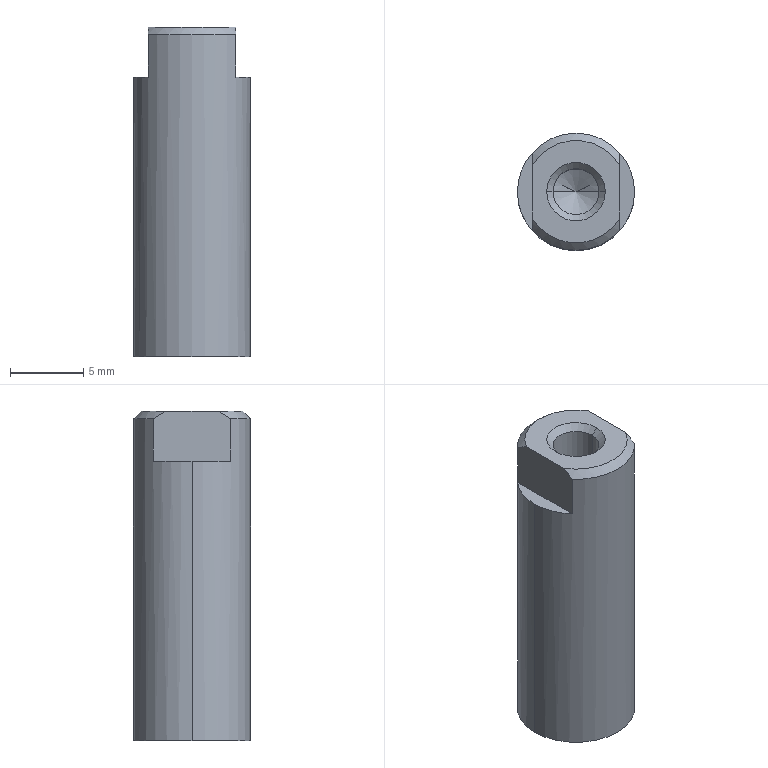Part | SolidWorks | features ICE 1, RevCut 1, Revolution 1 | 1 solid | 16 faces | box 8 x 8 x 22.5 mm | volume 1035 mm3 | cone 6 | plane 6 | cylinder 4 | commonest cylinder face diameters 3.14 x2 8 x2
STEP:
#1=CARTESIAN_POINT('',(0.,0.,-5.906));
#2=VERTEX_POINT('',#1);
#3=CARTESIAN_POINT('',(1.57,0.,-5.));
#4=VERTEX_POINT('',#3);
#5=CARTESIAN_POINT('',(0.,0.,-5.906));
#6=DIRECTION('',(0.866,0.,0.5));
#7=VECTOR('',#6,1000.);
#8=LINE('',#5,#7);
#9=EDGE_CURVE('',#2,#4,#8,.T.);
#10=ORIENTED_EDGE('',*,*,#9,.F.);
#11=CARTESIAN_POINT('',(-1.57,0.,-5.));
#12=VERTEX_POINT('',#11);
#13=CARTESIAN_POINT('',(0.,0.,-5.906));
#14=DIRECTION('',(-0.866,0.,0.5));
#15=VECTOR('',#14,1000.);
#16=LINE('',#13,#15);
#17=EDGE_CURVE('',#2,#12,#16,.T.);
#18=ORIENTED_EDGE('',*,*,#17,.T.);
#19=CARTESIAN_POINT('',(0.,0.,-5.));
#20=DIRECTION('',(0.,0.,1.));
#21=DIRECTION('',(1.,0.,0.));
#22=AXIS2_PLACEMENT_3D('',#19,#20,#21);
#23=CIRCLE('',#22,1.57);
#24=EDGE_CURVE('',#12,#4,#23,.T.);
#25=ORIENTED_EDGE('',*,*,#24,.T.);
#26=EDGE_LOOP('',(#10,#18,#25));
#27=FACE_OUTER_BOUND('',#26,.T.);
#28=CARTESIAN_POINT('',(0.,0.,994.094));
#29=DIRECTION('',(0.,0.,1.));
#30=DIRECTION('',(1.,0.,0.));
#31=AXIS2_PLACEMENT_3D('',#28,#29,#30);
#32=CONICAL_SURFACE('',#31,1732.051,1.047);
#33=ADVANCED_FACE('',(#27),#32,.F.);
#34=ORIENTED_EDGE('',*,*,#24,.F.);
#35=CARTESIAN_POINT('',(-1.57,0.,3.07));
#36=VERTEX_POINT('',#35);
#37=CARTESIAN_POINT('',(-1.57,0.,-5.906));
#38=DIRECTION('',(0.,0.,1.));
#39=VECTOR('',#38,1000.);
#40=LINE('',#37,#39);
#41=EDGE_CURVE('',#12,#36,#40,.T.);
#42=ORIENTED_EDGE('',*,*,#41,.T.);
#43=CARTESIAN_POINT('',(1.57,0.,3.07));
#44=VERTEX_POINT('',#43);
#45=CARTESIAN_POINT('',(0.,0.,3.07));
#46=DIRECTION('',(0.,0.,1.));
#47=DIRECTION('',(1.,0.,0.));
#48=AXIS2_PLACEMENT_3D('',#45,#46,#47);
#49=CIRCLE('',#48,1.57);
#50=EDGE_CURVE('',#36,#44,#49,.T.);
#51=ORIENTED_EDGE('',*,*,#50,.T.);
#52=CARTESIAN_POINT('',(1.57,0.,-5.906));
#53=DIRECTION('',(0.,0.,1.));
#54=VECTOR('',#53,1000.);
#55=LINE('',#52,#54);
#56=EDGE_CURVE('',#4,#44,#55,.T.);
#57=ORIENTED_EDGE('',*,*,#56,.F.);
#58=EDGE_LOOP('',(#34,#42,#51,#57));
#59=FACE_OUTER_BOUND('',#58,.T.);
#60=CARTESIAN_POINT('',(0.,0.,-5.906));
#61=DIRECTION('',(0.,0.,1.));
#62=DIRECTION('',(1.,0.,0.));
#63=AXIS2_PLACEMENT_3D('',#60,#61,#62);
#64=CYLINDRICAL_SURFACE('',#63,1.57);
#65=ADVANCED_FACE('',(#59),#64,.F.);
#66=ORIENTED_EDGE('',*,*,#50,.F.);
#67=CARTESIAN_POINT('',(-2.,0.,3.5));
#68=VERTEX_POINT('',#67);
#69=CARTESIAN_POINT('',(-1.57,0.,3.07));
#70=DIRECTION('',(-0.7071,0.,0.7071));
#71=VECTOR('',#70,1000.);
#72=LINE('',#69,#71);
#73=EDGE_CURVE('',#36,#68,#72,.T.);
#74=ORIENTED_EDGE('',*,*,#73,.T.);
#75=CARTESIAN_POINT('',(2.,0.,3.5));
#76=VERTEX_POINT('',#75);
#77=CARTESIAN_POINT('',(0.,0.,3.5));
#78=DIRECTION('',(0.,0.,1.));
#79=DIRECTION('',(-1.,0.,0.));
#80=AXIS2_PLACEMENT_3D('',#77,#78,#79);
#81=CIRCLE('',#80,2.);
#82=EDGE_CURVE('',#68,#76,#81,.T.);
#83=ORIENTED_EDGE('',*,*,#82,.T.);
#84=CARTESIAN_POINT('',(1.57,0.,3.07));
#85=DIRECTION('',(0.7071,0.,0.7071));
#86=VECTOR('',#85,1000.);
#87=LINE('',#84,#86);
#88=EDGE_CURVE('',#44,#76,#87,.T.);
#89=ORIENTED_EDGE('',*,*,#88,.F.);
#90=EDGE_LOOP('',(#66,#74,#83,#89));
#91=FACE_OUTER_BOUND('',#90,.T.);
#92=CARTESIAN_POINT('',(0.,0.,3.07));
#93=DIRECTION('',(0.,0.,1.));
#94=DIRECTION('',(1.,0.,0.));
#95=AXIS2_PLACEMENT_3D('',#92,#93,#94);
#96=CONICAL_SURFACE('',#95,1.57,0.7854);
#97=ADVANCED_FACE('',(#91),#96,.F.);
#98=CARTESIAN_POINT('',(4.,0.,-19.));
#99=VERTEX_POINT('',#98);
#100=CARTESIAN_POINT('',(-4.,0.,-19.));
#101=VERTEX_POINT('',#100);
#102=CARTESIAN_POINT('',(0.,0.,-19.));
#103=DIRECTION('',(0.,0.,1.));
#104=DIRECTION('',(1.,0.,0.));
#105=AXIS2_PLACEMENT_3D('',#102,#103,#104);
#106=CIRCLE('',#105,4.);
#107=EDGE_CURVE('',#99,#101,#106,.T.);
#108=ORIENTED_EDGE('',*,*,#107,.T.);
#109=CARTESIAN_POINT('',(-4.,0.,0.1));
#110=VERTEX_POINT('',#109);
#111=CARTESIAN_POINT('',(-4.,0.,-19.));
#112=DIRECTION('',(0.,0.,1.));
#113=VECTOR('',#112,1000.);
#114=LINE('',#111,#113);
#115=EDGE_CURVE('',#101,#110,#114,.T.);
#116=ORIENTED_EDGE('',*,*,#115,.T.);
#117=CARTESIAN_POINT('',(-3.,2.646,0.1));
#118=VERTEX_POINT('',#117);
#119=CARTESIAN_POINT('',(0.,0.,0.1));
#120=DIRECTION('',(0.,0.,1.));
#121=DIRECTION('',(1.,0.,0.));
#122=AXIS2_PLACEMENT_3D('',#119,#120,#121);
#123=CIRCLE('',#122,4.);
#124=EDGE_CURVE('',#118,#110,#123,.T.);
#125=ORIENTED_EDGE('',*,*,#124,.F.);
#126=CARTESIAN_POINT('',(-3.,2.646,3.));
#127=VERTEX_POINT('',#126);
#128=CARTESIAN_POINT('',(-3.,2.646,-19.));
#129=DIRECTION('',(0.,0.,1.));
#130=VECTOR('',#129,1000.);
#131=LINE('',#128,#130);
#132=EDGE_CURVE('',#118,#127,#131,.T.);
#133=ORIENTED_EDGE('',*,*,#132,.T.);
#134=CARTESIAN_POINT('',(3.,2.646,3.));
#135=VERTEX_POINT('',#134);
#136=CARTESIAN_POINT('',(0.,0.,3.));
#137=DIRECTION('',(0.,0.,1.));
#138=DIRECTION('',(1.,0.,0.));
#139=AXIS2_PLACEMENT_3D('',#136,#137,#138);
#140=CIRCLE('',#139,4.);
#141=EDGE_CURVE('',#135,#127,#140,.T.);
#142=ORIENTED_EDGE('',*,*,#141,.F.);
#143=CARTESIAN_POINT('',(3.,2.646,0.1));
#144=VERTEX_POINT('',#143);
#145=CARTESIAN_POINT('',(3.,2.646,-19.));
#146=DIRECTION('',(0.,0.,-1.));
#147=VECTOR('',#146,1000.);
#148=LINE('',#145,#147);
#149=EDGE_CURVE('',#135,#144,#148,.T.);
#150=ORIENTED_EDGE('',*,*,#149,.T.);
#151=CARTESIAN_POINT('',(4.,0.,0.1));
#152=VERTEX_POINT('',#151);
#153=CARTESIAN_POINT('',(0.,0.,0.1));
#154=DIRECTION('',(0.,0.,1.));
#155=DIRECTION('',(1.,0.,0.));
#156=AXIS2_PLACEMENT_3D('',#153,#154,#155);
#157=CIRCLE('',#156,4.);
#158=EDGE_CURVE('',#152,#144,#157,.T.);
#159=ORIENTED_EDGE('',*,*,#158,.F.);
#160=CARTESIAN_POINT('',(4.,0.,-19.));
#161=DIRECTION('',(0.,0.,1.));
#162=VECTOR('',#161,1000.);
#163=LINE('',#160,#162);
#164=EDGE_CURVE('',#99,#152,#163,.T.);
#165=ORIENTED_EDGE('',*,*,#164,.F.);
#166=EDGE_LOOP('',(#108,#116,#125,#133,#142,#150,#159,#165));
#167=FACE_OUTER_BOUND('',#166,.T.);
#168=CARTESIAN_POINT('',(0.,0.,-19.));
#169=DIRECTION('',(0.,0.,1.));
#170=DIRECTION('',(1.,0.,0.));
#171=AXIS2_PLACEMENT_3D('',#168,#169,#170);
#172=CYLINDRICAL_SURFACE('',#171,4.);
#173=ADVANCED_FACE('',(#167),#172,.T.);
#174=CARTESIAN_POINT('',(-3.,-1.803,3.5));
#175=VERTEX_POINT('',#174);
#176=CARTESIAN_POINT('',(3.,-1.803,3.5));
#177=VERTEX_POINT('',#176);
#178=CARTESIAN_POINT('',(0.,0.,3.5));
#179=DIRECTION('',(0.,0.,1.));
#180=DIRECTION('',(1.,0.,0.));
#181=AXIS2_PLACEMENT_3D('',#178,#179,#180);
#182=CIRCLE('',#181,3.5);
#183=EDGE_CURVE('',#175,#177,#182,.T.);
#184=ORIENTED_EDGE('',*,*,#183,.T.);
#185=CARTESIAN_POINT('',(3.,1.803,3.5));
#186=VERTEX_POINT('',#185);
#187=CARTESIAN_POINT('',(3.,6.,3.5));
#188=DIRECTION('',(0.,-1.,0.));
#189=VECTOR('',#188,1000.);
#190=LINE('',#187,#189);
#191=EDGE_CURVE('',#186,#177,#190,.T.);
#192=ORIENTED_EDGE('',*,*,#191,.F.);
#193=CARTESIAN_POINT('',(-3.,1.803,3.5));
#194=VERTEX_POINT('',#193);
#195=CARTESIAN_POINT('',(0.,0.,3.5));
#196=DIRECTION('',(0.,0.,1.));
#197=DIRECTION('',(1.,0.,0.));
#198=AXIS2_PLACEMENT_3D('',#195,#196,#197);
#199=CIRCLE('',#198,3.5);
#200=EDGE_CURVE('',#186,#194,#199,.T.);
#201=ORIENTED_EDGE('',*,*,#200,.T.);
#202=CARTESIAN_POINT('',(-3.,-6.,3.5));
#203=DIRECTION('',(0.,1.,0.));
#204=VECTOR('',#203,1000.);
#205=LINE('',#202,#204);
#206=EDGE_CURVE('',#175,#194,#205,.T.);
#207=ORIENTED_EDGE('',*,*,#206,.F.);
#208=EDGE_LOOP('',(#184,#192,#201,#207));
#209=FACE_OUTER_BOUND('',#208,.T.);
#210=CARTESIAN_POINT('',(0.,0.,3.5));
#211=DIRECTION('',(0.,0.,1.));
#212=DIRECTION('',(-1.,0.,0.));
#213=AXIS2_PLACEMENT_3D('',#210,#211,#212);
#214=CIRCLE('',#213,2.);
#215=EDGE_CURVE('',#76,#68,#214,.T.);
#216=ORIENTED_EDGE('',*,*,#215,.F.);
#217=ORIENTED_EDGE('',*,*,#82,.F.);
#218=EDGE_LOOP('',(#216,#217));
#219=FACE_BOUND('',#218,.T.);
#220=CARTESIAN_POINT('',(0.,0.,3.5));
#221=DIRECTION('',(0.,0.,-1.));
#222=DIRECTION('',(-1.,0.,0.));
#223=AXIS2_PLACEMENT_3D('',#220,#221,#222);
#224=PLANE('',#223);
#225=ADVANCED_FACE('',(#209,#219),#224,.F.);
#226=CARTESIAN_POINT('',(-3.,-2.646,3.));
#227=VERTEX_POINT('',#226);
#228=CARTESIAN_POINT('',(3.,-2.646,3.));
#229=VERTEX_POINT('',#228);
#230=CARTESIAN_POINT('',(0.,0.,3.));
#231=DIRECTION('',(0.,0.,1.));
#232=DIRECTION('',(1.,0.,0.));
#233=AXIS2_PLACEMENT_3D('',#230,#231,#232);
#234=CIRCLE('',#233,4.);
#235=EDGE_CURVE('',#227,#229,#234,.T.);
#236=ORIENTED_EDGE('',*,*,#235,.T.);
#237=CARTESIAN_POINT('',(3.,-2.646,3.));
#238=CARTESIAN_POINT('',(3.,-2.374,3.18));
#239=CARTESIAN_POINT('',(3.,-2.095,3.349));
#240=CARTESIAN_POINT('',(3.,-1.803,3.5));
#241=B_SPLINE_CURVE_WITH_KNOTS('',3,(#237,#238,#239,#240),.UNSPECIFIED.,.F.,.F.,(4,4),(0.007424,0.008405),.UNSPECIFIED.);
#242=EDGE_CURVE('',#229,#177,#241,.T.);
#243=ORIENTED_EDGE('',*,*,#242,.T.);
#244=ORIENTED_EDGE('',*,*,#183,.F.);
#245=CARTESIAN_POINT('',(-3.,-1.803,3.5));
#246=CARTESIAN_POINT('',(-3.,-2.092,3.351));
#247=CARTESIAN_POINT('',(-3.,-2.373,3.18));
#248=CARTESIAN_POINT('',(-3.,-2.646,3.));
#249=B_SPLINE_CURVE_WITH_KNOTS('',3,(#245,#246,#247,#248),.UNSPECIFIED.,.F.,.F.,(4,4),(0.01215,0.01313),.UNSPECIFIED.);
#250=EDGE_CURVE('',#175,#227,#249,.T.);
#251=ORIENTED_EDGE('',*,*,#250,.T.);
#252=EDGE_LOOP('',(#236,#243,#244,#251));
#253=FACE_OUTER_BOUND('',#252,.T.);
#254=CARTESIAN_POINT('',(0.,0.,3.));
#255=DIRECTION('',(0.,0.,-1.));
#256=DIRECTION('',(-1.,0.,0.));
#257=AXIS2_PLACEMENT_3D('',#254,#255,#256);
#258=CONICAL_SURFACE('',#257,4.,0.7854);
#259=ADVANCED_FACE('',(#253),#258,.T.);
#260=ORIENTED_EDGE('',*,*,#200,.F.);
#261=CARTESIAN_POINT('',(3.,1.803,3.5));
#262=CARTESIAN_POINT('',(3.,2.092,3.351));
#263=CARTESIAN_POINT('',(3.,2.373,3.18));
#264=CARTESIAN_POINT('',(3.,2.646,3.));
#265=B_SPLINE_CURVE_WITH_KNOTS('',3,(#261,#262,#263,#264),.UNSPECIFIED.,.F.,.F.,(4,4),(0.01215,0.01313),.UNSPECIFIED.);
#266=EDGE_CURVE('',#186,#135,#265,.T.);
#267=ORIENTED_EDGE('',*,*,#266,.T.);
#268=ORIENTED_EDGE('',*,*,#141,.T.);
#269=CARTESIAN_POINT('',(-3.,2.646,3.));
#270=CARTESIAN_POINT('',(-3.,2.374,3.18));
#271=CARTESIAN_POINT('',(-3.,2.095,3.349));
#272=CARTESIAN_POINT('',(-3.,1.803,3.5));
#273=B_SPLINE_CURVE_WITH_KNOTS('',3,(#269,#270,#271,#272),.UNSPECIFIED.,.F.,.F.,(4,4),(0.007424,0.008405),.UNSPECIFIED.);
#274=EDGE_CURVE('',#127,#194,#273,.T.);
#275=ORIENTED_EDGE('',*,*,#274,.T.);
#276=EDGE_LOOP('',(#260,#267,#268,#275));
#277=FACE_OUTER_BOUND('',#276,.T.);
#278=CARTESIAN_POINT('',(0.,0.,3.));
#279=DIRECTION('',(0.,0.,-1.));
#280=DIRECTION('',(-1.,0.,0.));
#281=AXIS2_PLACEMENT_3D('',#278,#279,#280);
#282=CONICAL_SURFACE('',#281,4.,0.7854);
#283=ADVANCED_FACE('',(#277),#282,.T.);
#284=ORIENTED_EDGE('',*,*,#115,.F.);
#285=CARTESIAN_POINT('',(0.,0.,-19.));
#286=DIRECTION('',(0.,0.,1.));
#287=DIRECTION('',(1.,0.,0.));
#288=AXIS2_PLACEMENT_3D('',#285,#286,#287);
#289=CIRCLE('',#288,4.);
#290=EDGE_CURVE('',#101,#99,#289,.T.);
#291=ORIENTED_EDGE('',*,*,#290,.T.);
#292=ORIENTED_EDGE('',*,*,#164,.T.);
#293=CARTESIAN_POINT('',(3.,-2.646,0.1));
#294=VERTEX_POINT('',#293);
#295=CARTESIAN_POINT('',(0.,0.,0.1));
#296=DIRECTION('',(0.,0.,1.));
#297=DIRECTION('',(1.,0.,0.));
#298=AXIS2_PLACEMENT_3D('',#295,#296,#297);
#299=CIRCLE('',#298,4.);
#300=EDGE_CURVE('',#294,#152,#299,.T.);
#301=ORIENTED_EDGE('',*,*,#300,.F.);
#302=CARTESIAN_POINT('',(3.,-2.646,-19.));
#303=DIRECTION('',(0.,0.,1.));
#304=VECTOR('',#303,1000.);
#305=LINE('',#302,#304);
#306=EDGE_CURVE('',#294,#229,#305,.T.);
#307=ORIENTED_EDGE('',*,*,#306,.T.);
#308=ORIENTED_EDGE('',*,*,#235,.F.);
#309=CARTESIAN_POINT('',(-3.,-2.646,0.1));
#310=VERTEX_POINT('',#309);
#311=CARTESIAN_POINT('',(-3.,-2.646,-19.));
#312=DIRECTION('',(0.,0.,-1.));
#313=VECTOR('',#312,1000.);
#314=LINE('',#311,#313);
#315=EDGE_CURVE('',#227,#310,#314,.T.);
#316=ORIENTED_EDGE('',*,*,#315,.T.);
#317=CARTESIAN_POINT('',(0.,0.,0.1));
#318=DIRECTION('',(0.,0.,1.));
#319=DIRECTION('',(1.,0.,0.));
#320=AXIS2_PLACEMENT_3D('',#317,#318,#319);
#321=CIRCLE('',#320,4.);
#322=EDGE_CURVE('',#110,#310,#321,.T.);
#323=ORIENTED_EDGE('',*,*,#322,.F.);
#324=EDGE_LOOP('',(#284,#291,#292,#301,#307,#308,#316,#323));
#325=FACE_OUTER_BOUND('',#324,.T.);
#326=CARTESIAN_POINT('',(0.,0.,-19.));
#327=DIRECTION('',(0.,0.,1.));
#328=DIRECTION('',(1.,0.,0.));
#329=AXIS2_PLACEMENT_3D('',#326,#327,#328);
#330=CYLINDRICAL_SURFACE('',#329,4.);
#331=ADVANCED_FACE('',(#325),#330,.T.);
#332=ORIENTED_EDGE('',*,*,#107,.F.);
#333=ORIENTED_EDGE('',*,*,#290,.F.);
#334=EDGE_LOOP('',(#332,#333));
#335=FACE_OUTER_BOUND('',#334,.T.);
#336=CARTESIAN_POINT('',(0.,4.,-19.));
#337=DIRECTION('',(0.,0.,1.));
#338=DIRECTION('',(1.,0.,0.));
#339=AXIS2_PLACEMENT_3D('',#336,#337,#338);
#340=PLANE('',#339);
#341=ADVANCED_FACE('',(#335),#340,.F.);
#342=ORIENTED_EDGE('',*,*,#300,.T.);
#343=ORIENTED_EDGE('',*,*,#158,.T.);
#344=CARTESIAN_POINT('',(3.,6.,0.1));
#345=DIRECTION('',(0.,-1.,0.));
#346=VECTOR('',#345,1000.);
#347=LINE('',#344,#346);
#348=EDGE_CURVE('',#144,#294,#347,.T.);
#349=ORIENTED_EDGE('',*,*,#348,.T.);
#350=EDGE_LOOP('',(#342,#343,#349));
#351=FACE_OUTER_BOUND('',#350,.T.);
#352=CARTESIAN_POINT('',(0.,0.,0.1));
#353=DIRECTION('',(0.,0.,1.));
#354=DIRECTION('',(1.,0.,0.));
#355=AXIS2_PLACEMENT_3D('',#352,#353,#354);
#356=PLANE('',#355);
#357=ADVANCED_FACE('',(#351),#356,.T.);
#358=ORIENTED_EDGE('',*,*,#306,.F.);
#359=ORIENTED_EDGE('',*,*,#348,.F.);
#360=ORIENTED_EDGE('',*,*,#149,.F.);
#361=ORIENTED_EDGE('',*,*,#266,.F.);
#362=ORIENTED_EDGE('',*,*,#191,.T.);
#363=ORIENTED_EDGE('',*,*,#242,.F.);
#364=EDGE_LOOP('',(#358,#359,#360,#361,#362,#363));
#365=FACE_OUTER_BOUND('',#364,.T.);
#366=CARTESIAN_POINT('',(3.,6.,0.1));
#367=DIRECTION('',(-1.,0.,0.));
#368=DIRECTION('',(0.,0.,1.));
#369=AXIS2_PLACEMENT_3D('',#366,#367,#368);
#370=PLANE('',#369);
#371=ADVANCED_FACE('',(#365),#370,.F.);
#372=ORIENTED_EDGE('',*,*,#132,.F.);
#373=CARTESIAN_POINT('',(-3.,-6.,0.1));
#374=DIRECTION('',(0.,1.,0.));
#375=VECTOR('',#374,1000.);
#376=LINE('',#373,#375);
#377=EDGE_CURVE('',#310,#118,#376,.T.);
#378=ORIENTED_EDGE('',*,*,#377,.F.);
#379=ORIENTED_EDGE('',*,*,#315,.F.);
#380=ORIENTED_EDGE('',*,*,#250,.F.);
#381=ORIENTED_EDGE('',*,*,#206,.T.);
#382=ORIENTED_EDGE('',*,*,#274,.F.);
#383=EDGE_LOOP('',(#372,#378,#379,#380,#381,#382));
#384=FACE_OUTER_BOUND('',#383,.T.);
#385=CARTESIAN_POINT('',(-3.,-6.,0.1));
#386=DIRECTION('',(1.,0.,0.));
#387=DIRECTION('',(0.,0.,-1.));
#388=AXIS2_PLACEMENT_3D('',#385,#386,#387);
#389=PLANE('',#388);
#390=ADVANCED_FACE('',(#384),#389,.F.);
#391=ORIENTED_EDGE('',*,*,#124,.T.);
#392=ORIENTED_EDGE('',*,*,#322,.T.);
#393=ORIENTED_EDGE('',*,*,#377,.T.);
#394=EDGE_LOOP('',(#391,#392,#393));
#395=FACE_OUTER_BOUND('',#394,.T.);
#396=CARTESIAN_POINT('',(0.,0.,0.1));
#397=DIRECTION('',(0.,0.,1.));
#398=DIRECTION('',(1.,0.,0.));
#399=AXIS2_PLACEMENT_3D('',#396,#397,#398);
#400=PLANE('',#399);
#401=ADVANCED_FACE('',(#395),#400,.T.);
#402=ORIENTED_EDGE('',*,*,#73,.F.);
#403=CARTESIAN_POINT('',(0.,0.,3.07));
#404=DIRECTION('',(0.,0.,1.));
#405=DIRECTION('',(1.,0.,0.));
#406=AXIS2_PLACEMENT_3D('',#403,#404,#405);
#407=CIRCLE('',#406,1.57);
#408=EDGE_CURVE('',#44,#36,#407,.T.);
#409=ORIENTED_EDGE('',*,*,#408,.F.);
#410=ORIENTED_EDGE('',*,*,#88,.T.);
#411=ORIENTED_EDGE('',*,*,#215,.T.);
#412=EDGE_LOOP('',(#402,#409,#410,#411));
#413=FACE_OUTER_BOUND('',#412,.T.);
#414=CARTESIAN_POINT('',(0.,0.,3.07));
#415=DIRECTION('',(0.,0.,1.));
#416=DIRECTION('',(1.,0.,0.));
#417=AXIS2_PLACEMENT_3D('',#414,#415,#416);
#418=CONICAL_SURFACE('',#417,1.57,0.7854);
#419=ADVANCED_FACE('',(#413),#418,.F.);
#420=ORIENTED_EDGE('',*,*,#41,.F.);
#421=CARTESIAN_POINT('',(0.,0.,-5.));
#422=DIRECTION('',(0.,0.,1.));
#423=DIRECTION('',(1.,0.,0.));
#424=AXIS2_PLACEMENT_3D('',#421,#422,#423);
#425=CIRCLE('',#424,1.57);
#426=EDGE_CURVE('',#4,#12,#425,.T.);
#427=ORIENTED_EDGE('',*,*,#426,.F.);
#428=ORIENTED_EDGE('',*,*,#56,.T.);
#429=ORIENTED_EDGE('',*,*,#408,.T.);
#430=EDGE_LOOP('',(#420,#427,#428,#429));
#431=FACE_OUTER_BOUND('',#430,.T.);
#432=CARTESIAN_POINT('',(0.,0.,-5.906));
#433=DIRECTION('',(0.,0.,1.));
#434=DIRECTION('',(1.,0.,0.));
#435=AXIS2_PLACEMENT_3D('',#432,#433,#434);
#436=CYLINDRICAL_SURFACE('',#435,1.57);
#437=ADVANCED_FACE('',(#431),#436,.F.);
#438=ORIENTED_EDGE('',*,*,#17,.F.);
#439=ORIENTED_EDGE('',*,*,#9,.T.);
#440=ORIENTED_EDGE('',*,*,#426,.T.);
#441=EDGE_LOOP('',(#438,#439,#440));
#442=FACE_OUTER_BOUND('',#441,.T.);
#443=CARTESIAN_POINT('',(0.,0.,994.094));
#444=DIRECTION('',(0.,0.,1.));
#445=DIRECTION('',(1.,0.,0.));
#446=AXIS2_PLACEMENT_3D('',#443,#444,#445);
#447=CONICAL_SURFACE('',#446,1732.051,1.047);
#448=ADVANCED_FACE('',(#442),#447,.F.);
#449=CLOSED_SHELL('',(#33,#65,#97,#173,#225,#259,#283,#331,#341,#357,#371,#390,#401,#419,#437,#448));
#450=MANIFOLD_SOLID_BREP('',#449);
#451=CARTESIAN_POINT('',(0.,0.,0.));
#452=DIRECTION('',(0.,0.,1.));
#453=DIRECTION('',(1.,0.,0.));
#454=AXIS2_PLACEMENT_3D('',#451,#452,#453);
#455=(LENGTH_UNIT()NAMED_UNIT(*)SI_UNIT(.MILLI.,.METRE.));
#456=UNCERTAINTY_MEASURE_WITH_UNIT(LENGTH_MEASURE(0.00001),#455,'','');
#457=(NAMED_UNIT(*)PLANE_ANGLE_UNIT()SI_UNIT($,.RADIAN.));
#458=(NAMED_UNIT(*)SI_UNIT($,.STERADIAN.)SOLID_ANGLE_UNIT());
#459=(GEOMETRIC_REPRESENTATION_CONTEXT(3)GLOBAL_UNCERTAINTY_ASSIGNED_CONTEXT((#456))GLOBAL_UNIT_ASSIGNED_CONTEXT((#455,#457,#458))REPRESENTATION_CONTEXT('',''));
#460=ADVANCED_BREP_SHAPE_REPRESENTATION('',(#450,#454),#459);